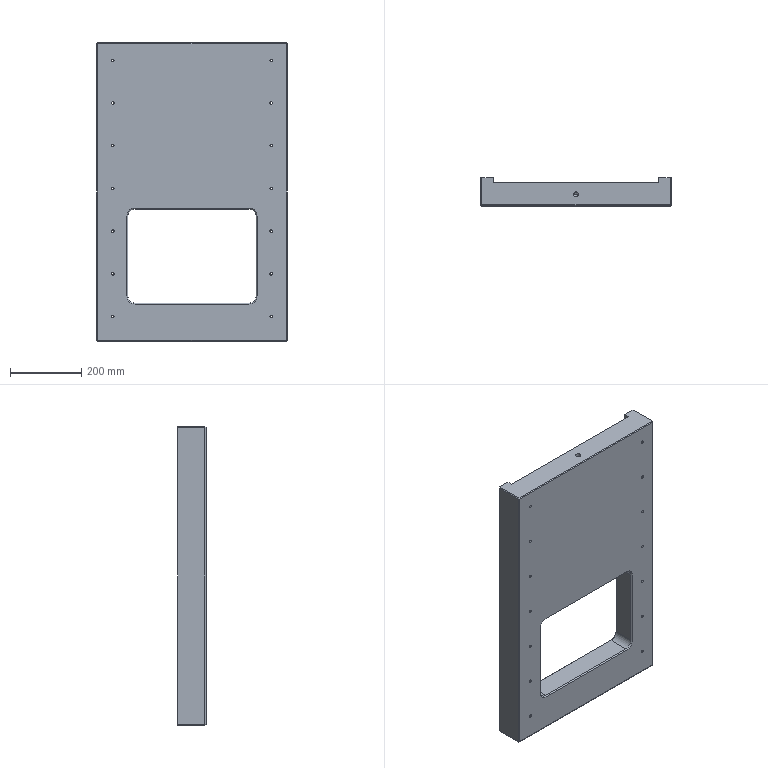Part | NX | features BREP 1 | 1 solid | 230 faces | box 535 x 79 x 840 mm | volume 23765456 mm3 | cylinder 116 | cone 64 | plane 50 | commonest cylinder face diameters 3.3 x48 7 x28 15 x28 2.5 x4 14 x4 40 x4